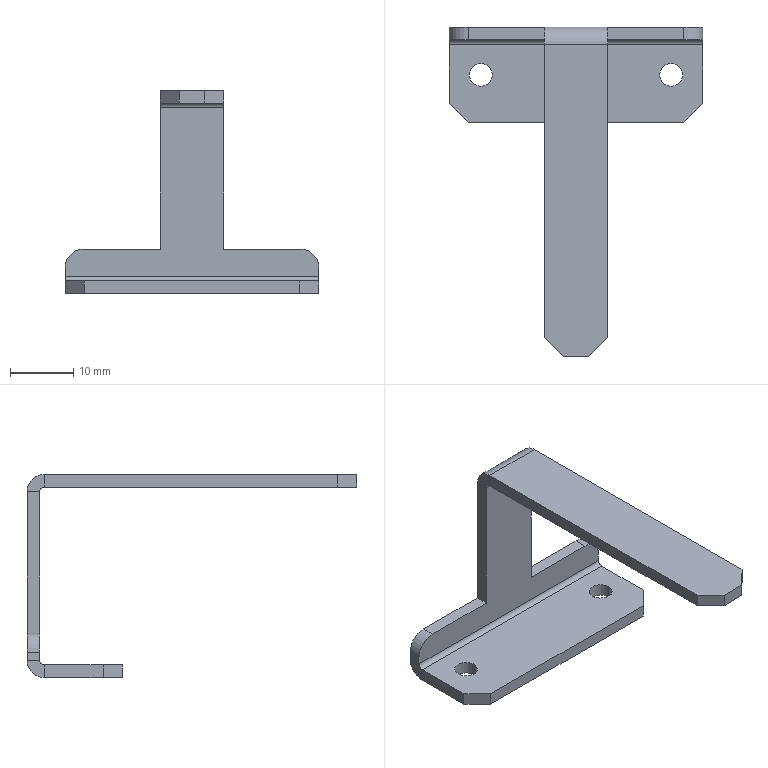Part | SolidWorks | features BaseBody 1 | 1 solid | 36 faces | box 40 x 52 x 32 mm | volume 2941 mm3 | plane 26 | cylinder 10 | commonest cylinder face diameters 3.6 x4 1.473 x2 5.473 x2 6 x2
STEP:
#1=CARTESIAN_POINT('',(-16.8,0.,-2.));
#2=VERTEX_POINT('',#1);
#3=CARTESIAN_POINT('',(-13.2,0.,-2.));
#4=VERTEX_POINT('',#3);
#5=CARTESIAN_POINT('',(-15.,0.,-2.));
#6=DIRECTION('',(0.,0.,1.));
#7=DIRECTION('',(1.,0.,0.));
#8=AXIS2_PLACEMENT_3D('',#5,#6,#7);
#9=CIRCLE('',#8,1.8);
#10=EDGE_CURVE('',#2,#4,#9,.T.);
#11=ORIENTED_EDGE('',*,*,#10,.F.);
#12=CARTESIAN_POINT('',(-16.8,0.,0.));
#13=VERTEX_POINT('',#12);
#14=CARTESIAN_POINT('',(-16.8,0.,0.));
#15=DIRECTION('',(0.,0.,1.));
#16=VECTOR('',#15,1000.);
#17=LINE('',#14,#16);
#18=EDGE_CURVE('',#2,#13,#17,.T.);
#19=ORIENTED_EDGE('',*,*,#18,.T.);
#20=CARTESIAN_POINT('',(-13.2,0.,0.));
#21=VERTEX_POINT('',#20);
#22=CARTESIAN_POINT('',(-15.,0.,0.));
#23=DIRECTION('',(0.,0.,1.));
#24=DIRECTION('',(1.,0.,0.));
#25=AXIS2_PLACEMENT_3D('',#22,#23,#24);
#26=CIRCLE('',#25,1.8);
#27=EDGE_CURVE('',#13,#21,#26,.T.);
#28=ORIENTED_EDGE('',*,*,#27,.T.);
#29=CARTESIAN_POINT('',(-13.2,0.,0.));
#30=DIRECTION('',(0.,0.,1.));
#31=VECTOR('',#30,1000.);
#32=LINE('',#29,#31);
#33=EDGE_CURVE('',#4,#21,#32,.T.);
#34=ORIENTED_EDGE('',*,*,#33,.F.);
#35=EDGE_LOOP('',(#11,#19,#28,#34));
#36=FACE_OUTER_BOUND('',#35,.T.);
#37=CARTESIAN_POINT('',(-15.,0.,0.));
#38=DIRECTION('',(0.,0.,1.));
#39=DIRECTION('',(1.,0.,0.));
#40=AXIS2_PLACEMENT_3D('',#37,#38,#39);
#41=CYLINDRICAL_SURFACE('',#40,1.8);
#42=ADVANCED_FACE('',(#36),#41,.F.);
#43=CARTESIAN_POINT('',(13.2,0.,-2.));
#44=VERTEX_POINT('',#43);
#45=CARTESIAN_POINT('',(16.8,0.,-2.));
#46=VERTEX_POINT('',#45);
#47=CARTESIAN_POINT('',(15.,0.,-2.));
#48=DIRECTION('',(0.,0.,1.));
#49=DIRECTION('',(1.,0.,0.));
#50=AXIS2_PLACEMENT_3D('',#47,#48,#49);
#51=CIRCLE('',#50,1.8);
#52=EDGE_CURVE('',#44,#46,#51,.T.);
#53=ORIENTED_EDGE('',*,*,#52,.F.);
#54=CARTESIAN_POINT('',(13.2,0.,0.));
#55=VERTEX_POINT('',#54);
#56=CARTESIAN_POINT('',(13.2,0.,0.));
#57=DIRECTION('',(0.,0.,1.));
#58=VECTOR('',#57,1000.);
#59=LINE('',#56,#58);
#60=EDGE_CURVE('',#44,#55,#59,.T.);
#61=ORIENTED_EDGE('',*,*,#60,.T.);
#62=CARTESIAN_POINT('',(16.8,0.,0.));
#63=VERTEX_POINT('',#62);
#64=CARTESIAN_POINT('',(15.,0.,0.));
#65=DIRECTION('',(0.,0.,1.));
#66=DIRECTION('',(1.,0.,0.));
#67=AXIS2_PLACEMENT_3D('',#64,#65,#66);
#68=CIRCLE('',#67,1.8);
#69=EDGE_CURVE('',#55,#63,#68,.T.);
#70=ORIENTED_EDGE('',*,*,#69,.T.);
#71=CARTESIAN_POINT('',(16.8,0.,0.));
#72=DIRECTION('',(0.,0.,1.));
#73=VECTOR('',#72,1000.);
#74=LINE('',#71,#73);
#75=EDGE_CURVE('',#46,#63,#74,.T.);
#76=ORIENTED_EDGE('',*,*,#75,.F.);
#77=EDGE_LOOP('',(#53,#61,#70,#76));
#78=FACE_OUTER_BOUND('',#77,.T.);
#79=CARTESIAN_POINT('',(15.,0.,0.));
#80=DIRECTION('',(0.,0.,1.));
#81=DIRECTION('',(1.,0.,0.));
#82=AXIS2_PLACEMENT_3D('',#79,#80,#81);
#83=CYLINDRICAL_SURFACE('',#82,1.8);
#84=ADVANCED_FACE('',(#78),#83,.F.);
#85=CARTESIAN_POINT('',(-5.,4.763,28.));
#86=VERTEX_POINT('',#85);
#87=CARTESIAN_POINT('',(-5.,-41.5,28.));
#88=VERTEX_POINT('',#87);
#89=CARTESIAN_POINT('',(-5.,0.,28.));
#90=DIRECTION('',(0.,-1.,0.));
#91=VECTOR('',#90,1000.);
#92=LINE('',#89,#91);
#93=EDGE_CURVE('',#86,#88,#92,.T.);
#94=ORIENTED_EDGE('',*,*,#93,.T.);
#95=CARTESIAN_POINT('',(-5.,-41.5,30.));
#96=VERTEX_POINT('',#95);
#97=CARTESIAN_POINT('',(-5.,-41.5,5.));
#98=DIRECTION('',(0.,0.,1.));
#99=VECTOR('',#98,1000.);
#100=LINE('',#97,#99);
#101=EDGE_CURVE('',#88,#96,#100,.T.);
#102=ORIENTED_EDGE('',*,*,#101,.T.);
#103=CARTESIAN_POINT('',(-5.,4.763,30.));
#104=VERTEX_POINT('',#103);
#105=CARTESIAN_POINT('',(-5.,-44.5,30.));
#106=DIRECTION('',(0.,-1.,0.));
#107=VECTOR('',#106,1000.);
#108=LINE('',#105,#107);
#109=EDGE_CURVE('',#104,#96,#108,.T.);
#110=ORIENTED_EDGE('',*,*,#109,.F.);
#111=CARTESIAN_POINT('',(-5.,4.763,30.));
#112=DIRECTION('',(0.,0.,-1.));
#113=VECTOR('',#112,1000.);
#114=LINE('',#111,#113);
#115=EDGE_CURVE('',#104,#86,#114,.T.);
#116=ORIENTED_EDGE('',*,*,#115,.T.);
#117=EDGE_LOOP('',(#94,#102,#110,#116));
#118=FACE_OUTER_BOUND('',#117,.T.);
#119=CARTESIAN_POINT('',(-5.,-44.5,5.));
#120=DIRECTION('',(-1.,0.,0.));
#121=DIRECTION('',(0.,-1.,0.));
#122=AXIS2_PLACEMENT_3D('',#119,#120,#121);
#123=PLANE('',#122);
#124=ADVANCED_FACE('',(#118),#123,.T.);
#125=CARTESIAN_POINT('',(-5.,5.5,5.));
#126=VERTEX_POINT('',#125);
#127=CARTESIAN_POINT('',(-5.,5.5,27.263));
#128=VERTEX_POINT('',#127);
#129=CARTESIAN_POINT('',(-5.,5.5,0.));
#130=DIRECTION('',(0.,0.,1.));
#131=VECTOR('',#130,1000.);
#132=LINE('',#129,#131);
#133=EDGE_CURVE('',#126,#128,#132,.T.);
#134=ORIENTED_EDGE('',*,*,#133,.T.);
#135=CARTESIAN_POINT('',(-5.,7.5,27.263));
#136=VERTEX_POINT('',#135);
#137=CARTESIAN_POINT('',(-5.,5.5,27.263));
#138=DIRECTION('',(0.,1.,0.));
#139=VECTOR('',#138,1000.);
#140=LINE('',#137,#139);
#141=EDGE_CURVE('',#128,#136,#140,.T.);
#142=ORIENTED_EDGE('',*,*,#141,.T.);
#143=CARTESIAN_POINT('',(-5.,7.5,5.));
#144=VERTEX_POINT('',#143);
#145=CARTESIAN_POINT('',(-5.,7.5,0.));
#146=DIRECTION('',(0.,0.,1.));
#147=VECTOR('',#146,1000.);
#148=LINE('',#145,#147);
#149=EDGE_CURVE('',#144,#136,#148,.T.);
#150=ORIENTED_EDGE('',*,*,#149,.F.);
#151=CARTESIAN_POINT('',(-5.,-44.5,5.));
#152=DIRECTION('',(0.,-1.,0.));
#153=VECTOR('',#152,1000.);
#154=LINE('',#151,#153);
#155=EDGE_CURVE('',#144,#126,#154,.T.);
#156=ORIENTED_EDGE('',*,*,#155,.T.);
#157=EDGE_LOOP('',(#134,#142,#150,#156));
#158=FACE_OUTER_BOUND('',#157,.T.);
#159=CARTESIAN_POINT('',(-5.,-44.5,5.));
#160=DIRECTION('',(-1.,0.,0.));
#161=DIRECTION('',(0.,-1.,0.));
#162=AXIS2_PLACEMENT_3D('',#159,#160,#161);
#163=PLANE('',#162);
#164=ADVANCED_FACE('',(#158),#163,.T.);
#165=CARTESIAN_POINT('',(5.,-41.5,30.));
#166=VERTEX_POINT('',#165);
#167=CARTESIAN_POINT('',(5.,4.763,30.));
#168=VERTEX_POINT('',#167);
#169=CARTESIAN_POINT('',(5.,-44.5,30.));
#170=DIRECTION('',(0.,1.,0.));
#171=VECTOR('',#170,1000.);
#172=LINE('',#169,#171);
#173=EDGE_CURVE('',#166,#168,#172,.T.);
#174=ORIENTED_EDGE('',*,*,#173,.F.);
#175=CARTESIAN_POINT('',(5.,-41.5,28.));
#176=VERTEX_POINT('',#175);
#177=CARTESIAN_POINT('',(5.,-41.5,5.));
#178=DIRECTION('',(0.,0.,-1.));
#179=VECTOR('',#178,1000.);
#180=LINE('',#177,#179);
#181=EDGE_CURVE('',#166,#176,#180,.T.);
#182=ORIENTED_EDGE('',*,*,#181,.T.);
#183=CARTESIAN_POINT('',(5.,4.763,28.));
#184=VERTEX_POINT('',#183);
#185=CARTESIAN_POINT('',(5.,0.,28.));
#186=DIRECTION('',(0.,1.,0.));
#187=VECTOR('',#186,1000.);
#188=LINE('',#185,#187);
#189=EDGE_CURVE('',#176,#184,#188,.T.);
#190=ORIENTED_EDGE('',*,*,#189,.T.);
#191=CARTESIAN_POINT('',(5.,4.763,28.));
#192=DIRECTION('',(0.,0.,1.));
#193=VECTOR('',#192,1000.);
#194=LINE('',#191,#193);
#195=EDGE_CURVE('',#184,#168,#194,.T.);
#196=ORIENTED_EDGE('',*,*,#195,.T.);
#197=EDGE_LOOP('',(#174,#182,#190,#196));
#198=FACE_OUTER_BOUND('',#197,.T.);
#199=CARTESIAN_POINT('',(5.,-44.5,5.));
#200=DIRECTION('',(1.,0.,0.));
#201=DIRECTION('',(0.,0.,-1.));
#202=AXIS2_PLACEMENT_3D('',#199,#200,#201);
#203=PLANE('',#202);
#204=ADVANCED_FACE('',(#198),#203,.T.);
#205=CARTESIAN_POINT('',(5.,7.5,27.263));
#206=VERTEX_POINT('',#205);
#207=CARTESIAN_POINT('',(5.,7.5,5.));
#208=VERTEX_POINT('',#207);
#209=CARTESIAN_POINT('',(5.,7.5,0.));
#210=DIRECTION('',(0.,0.,-1.));
#211=VECTOR('',#210,1000.);
#212=LINE('',#209,#211);
#213=EDGE_CURVE('',#206,#208,#212,.T.);
#214=ORIENTED_EDGE('',*,*,#213,.F.);
#215=CARTESIAN_POINT('',(5.,5.5,27.263));
#216=VERTEX_POINT('',#215);
#217=CARTESIAN_POINT('',(5.,7.5,27.263));
#218=DIRECTION('',(0.,-1.,0.));
#219=VECTOR('',#218,1000.);
#220=LINE('',#217,#219);
#221=EDGE_CURVE('',#206,#216,#220,.T.);
#222=ORIENTED_EDGE('',*,*,#221,.T.);
#223=CARTESIAN_POINT('',(5.,5.5,5.));
#224=VERTEX_POINT('',#223);
#225=CARTESIAN_POINT('',(5.,5.5,0.));
#226=DIRECTION('',(0.,0.,-1.));
#227=VECTOR('',#226,1000.);
#228=LINE('',#225,#227);
#229=EDGE_CURVE('',#216,#224,#228,.T.);
#230=ORIENTED_EDGE('',*,*,#229,.T.);
#231=CARTESIAN_POINT('',(5.,-44.5,5.));
#232=DIRECTION('',(0.,1.,0.));
#233=VECTOR('',#232,1000.);
#234=LINE('',#231,#233);
#235=EDGE_CURVE('',#224,#208,#234,.T.);
#236=ORIENTED_EDGE('',*,*,#235,.T.);
#237=EDGE_LOOP('',(#214,#222,#230,#236));
#238=FACE_OUTER_BOUND('',#237,.T.);
#239=CARTESIAN_POINT('',(5.,-44.5,5.));
#240=DIRECTION('',(1.,0.,0.));
#241=DIRECTION('',(0.,0.,-1.));
#242=AXIS2_PLACEMENT_3D('',#239,#240,#241);
#243=PLANE('',#242);
#244=ADVANCED_FACE('',(#238),#243,.T.);
#245=CARTESIAN_POINT('',(17.,7.5,5.));
#246=VERTEX_POINT('',#245);
#247=CARTESIAN_POINT('',(0.,7.5,5.));
#248=DIRECTION('',(1.,0.,0.));
#249=VECTOR('',#248,1000.);
#250=LINE('',#247,#249);
#251=EDGE_CURVE('',#208,#246,#250,.T.);
#252=ORIENTED_EDGE('',*,*,#251,.T.);
#253=CARTESIAN_POINT('',(20.,7.5,2.));
#254=VERTEX_POINT('',#253);
#255=CARTESIAN_POINT('',(17.,7.5,2.));
#256=DIRECTION('',(0.,1.,0.));
#257=DIRECTION('',(0.,0.,1.));
#258=AXIS2_PLACEMENT_3D('',#255,#256,#257);
#259=CIRCLE('',#258,3.);
#260=EDGE_CURVE('',#246,#254,#259,.T.);
#261=ORIENTED_EDGE('',*,*,#260,.T.);
#262=CARTESIAN_POINT('',(20.,7.5,0.7366));
#263=VERTEX_POINT('',#262);
#264=CARTESIAN_POINT('',(20.,7.5,28.));
#265=DIRECTION('',(0.,0.,1.));
#266=VECTOR('',#265,1000.);
#267=LINE('',#264,#266);
#268=EDGE_CURVE('',#263,#254,#267,.T.);
#269=ORIENTED_EDGE('',*,*,#268,.F.);
#270=CARTESIAN_POINT('',(-20.,7.5,0.7366));
#271=VERTEX_POINT('',#270);
#272=CARTESIAN_POINT('',(0.,7.5,0.7366));
#273=DIRECTION('',(-1.,0.,0.));
#274=VECTOR('',#273,1000.);
#275=LINE('',#272,#274);
#276=EDGE_CURVE('',#263,#271,#275,.T.);
#277=ORIENTED_EDGE('',*,*,#276,.T.);
#278=CARTESIAN_POINT('',(-20.,7.5,2.));
#279=VERTEX_POINT('',#278);
#280=CARTESIAN_POINT('',(-20.,7.5,0.));
#281=DIRECTION('',(0.,0.,-1.));
#282=VECTOR('',#281,1000.);
#283=LINE('',#280,#282);
#284=EDGE_CURVE('',#279,#271,#283,.T.);
#285=ORIENTED_EDGE('',*,*,#284,.F.);
#286=CARTESIAN_POINT('',(-17.,7.5,5.));
#287=VERTEX_POINT('',#286);
#288=CARTESIAN_POINT('',(-17.,7.5,2.));
#289=DIRECTION('',(0.,1.,0.));
#290=DIRECTION('',(0.,0.,1.));
#291=AXIS2_PLACEMENT_3D('',#288,#289,#290);
#292=CIRCLE('',#291,3.);
#293=EDGE_CURVE('',#279,#287,#292,.T.);
#294=ORIENTED_EDGE('',*,*,#293,.T.);
#295=CARTESIAN_POINT('',(0.,7.5,5.));
#296=DIRECTION('',(1.,0.,0.));
#297=VECTOR('',#296,1000.);
#298=LINE('',#295,#297);
#299=EDGE_CURVE('',#287,#144,#298,.T.);
#300=ORIENTED_EDGE('',*,*,#299,.T.);
#301=ORIENTED_EDGE('',*,*,#149,.T.);
#302=CARTESIAN_POINT('',(-20.,7.5,27.263));
#303=DIRECTION('',(1.,0.,0.));
#304=VECTOR('',#303,1000.);
#305=LINE('',#302,#304);
#306=EDGE_CURVE('',#136,#206,#305,.T.);
#307=ORIENTED_EDGE('',*,*,#306,.T.);
#308=ORIENTED_EDGE('',*,*,#213,.T.);
#309=EDGE_LOOP('',(#252,#261,#269,#277,#285,#294,#300,#301,#307,#308));
#310=FACE_OUTER_BOUND('',#309,.T.);
#311=CARTESIAN_POINT('',(0.,7.5,0.));
#312=DIRECTION('',(0.,1.,0.));
#313=DIRECTION('',(0.,0.,1.));
#314=AXIS2_PLACEMENT_3D('',#311,#312,#313);
#315=PLANE('',#314);
#316=ADVANCED_FACE('',(#310),#315,.T.);
#317=CARTESIAN_POINT('',(20.,5.5,0.7366));
#318=VERTEX_POINT('',#317);
#319=CARTESIAN_POINT('',(20.,5.5,2.));
#320=VERTEX_POINT('',#319);
#321=CARTESIAN_POINT('',(20.,5.5,0.));
#322=DIRECTION('',(0.,0.,1.));
#323=VECTOR('',#322,1000.);
#324=LINE('',#321,#323);
#325=EDGE_CURVE('',#318,#320,#324,.T.);
#326=ORIENTED_EDGE('',*,*,#325,.T.);
#327=CARTESIAN_POINT('',(17.,5.5,5.));
#328=VERTEX_POINT('',#327);
#329=CARTESIAN_POINT('',(17.,5.5,2.));
#330=DIRECTION('',(0.,-1.,0.));
#331=DIRECTION('',(0.,0.,1.));
#332=AXIS2_PLACEMENT_3D('',#329,#330,#331);
#333=CIRCLE('',#332,3.);
#334=EDGE_CURVE('',#320,#328,#333,.T.);
#335=ORIENTED_EDGE('',*,*,#334,.T.);
#336=CARTESIAN_POINT('',(0.,5.5,5.));
#337=DIRECTION('',(1.,0.,0.));
#338=VECTOR('',#337,1000.);
#339=LINE('',#336,#338);
#340=EDGE_CURVE('',#224,#328,#339,.T.);
#341=ORIENTED_EDGE('',*,*,#340,.F.);
#342=ORIENTED_EDGE('',*,*,#229,.F.);
#343=CARTESIAN_POINT('',(-20.,5.5,27.263));
#344=DIRECTION('',(1.,0.,0.));
#345=VECTOR('',#344,1000.);
#346=LINE('',#343,#345);
#347=EDGE_CURVE('',#128,#216,#346,.T.);
#348=ORIENTED_EDGE('',*,*,#347,.F.);
#349=ORIENTED_EDGE('',*,*,#133,.F.);
#350=CARTESIAN_POINT('',(-17.,5.5,5.));
#351=VERTEX_POINT('',#350);
#352=CARTESIAN_POINT('',(0.,5.5,5.));
#353=DIRECTION('',(1.,0.,0.));
#354=VECTOR('',#353,1000.);
#355=LINE('',#352,#354);
#356=EDGE_CURVE('',#351,#126,#355,.T.);
#357=ORIENTED_EDGE('',*,*,#356,.F.);
#358=CARTESIAN_POINT('',(-20.,5.5,2.));
#359=VERTEX_POINT('',#358);
#360=CARTESIAN_POINT('',(-17.,5.5,2.));
#361=DIRECTION('',(0.,-1.,0.));
#362=DIRECTION('',(0.,0.,1.));
#363=AXIS2_PLACEMENT_3D('',#360,#361,#362);
#364=CIRCLE('',#363,3.);
#365=EDGE_CURVE('',#351,#359,#364,.T.);
#366=ORIENTED_EDGE('',*,*,#365,.T.);
#367=CARTESIAN_POINT('',(-20.,5.5,0.7366));
#368=VERTEX_POINT('',#367);
#369=CARTESIAN_POINT('',(-20.,5.5,0.));
#370=DIRECTION('',(0.,0.,-1.));
#371=VECTOR('',#370,1000.);
#372=LINE('',#369,#371);
#373=EDGE_CURVE('',#359,#368,#372,.T.);
#374=ORIENTED_EDGE('',*,*,#373,.T.);
#375=CARTESIAN_POINT('',(20.,5.5,0.7366));
#376=DIRECTION('',(-1.,0.,0.));
#377=VECTOR('',#376,1000.);
#378=LINE('',#375,#377);
#379=EDGE_CURVE('',#318,#368,#378,.T.);
#380=ORIENTED_EDGE('',*,*,#379,.F.);
#381=EDGE_LOOP('',(#326,#335,#341,#342,#348,#349,#357,#366,#374,#380));
#382=FACE_OUTER_BOUND('',#381,.T.);
#383=CARTESIAN_POINT('',(0.,5.5,0.));
#384=DIRECTION('',(0.,1.,0.));
#385=DIRECTION('',(0.,0.,1.));
#386=AXIS2_PLACEMENT_3D('',#383,#384,#385);
#387=PLANE('',#386);
#388=ADVANCED_FACE('',(#382),#387,.F.);
#389=ORIENTED_EDGE('',*,*,#306,.F.);
#390=CARTESIAN_POINT('',(-5.,4.763,27.263));
#391=DIRECTION('',(1.,0.,0.));
#392=DIRECTION('',(0.,-1.,0.));
#393=AXIS2_PLACEMENT_3D('',#390,#391,#392);
#394=CIRCLE('',#393,2.737);
#395=EDGE_CURVE('',#136,#104,#394,.T.);
#396=ORIENTED_EDGE('',*,*,#395,.T.);
#397=CARTESIAN_POINT('',(0.,4.763,30.));
#398=DIRECTION('',(-1.,0.,0.));
#399=VECTOR('',#398,1000.);
#400=LINE('',#397,#399);
#401=EDGE_CURVE('',#168,#104,#400,.T.);
#402=ORIENTED_EDGE('',*,*,#401,.F.);
#403=CARTESIAN_POINT('',(5.,4.763,27.263));
#404=DIRECTION('',(-1.,0.,0.));
#405=DIRECTION('',(0.,0.,-1.));
#406=AXIS2_PLACEMENT_3D('',#403,#404,#405);
#407=CIRCLE('',#406,2.737);
#408=EDGE_CURVE('',#168,#206,#407,.T.);
#409=ORIENTED_EDGE('',*,*,#408,.T.);
#410=EDGE_LOOP('',(#389,#396,#402,#409));
#411=FACE_OUTER_BOUND('',#410,.T.);
#412=CARTESIAN_POINT('',(-20.,4.763,27.263));
#413=DIRECTION('',(-1.,0.,0.));
#414=DIRECTION('',(0.,0.,1.));
#415=AXIS2_PLACEMENT_3D('',#412,#413,#414);
#416=CYLINDRICAL_SURFACE('',#415,2.737);
#417=ADVANCED_FACE('',(#411),#416,.T.);
#418=CARTESIAN_POINT('',(-5.,4.763,27.263));
#419=DIRECTION('',(1.,0.,0.));
#420=DIRECTION('',(0.,-1.,0.));
#421=AXIS2_PLACEMENT_3D('',#418,#419,#420);
#422=CIRCLE('',#421,0.7366);
#423=EDGE_CURVE('',#128,#86,#422,.T.);
#424=ORIENTED_EDGE('',*,*,#423,.F.);
#425=ORIENTED_EDGE('',*,*,#347,.T.);
#426=CARTESIAN_POINT('',(5.,4.763,27.263));
#427=DIRECTION('',(-1.,0.,0.));
#428=DIRECTION('',(0.,0.,-1.));
#429=AXIS2_PLACEMENT_3D('',#426,#427,#428);
#430=CIRCLE('',#429,0.7366);
#431=EDGE_CURVE('',#184,#216,#430,.T.);
#432=ORIENTED_EDGE('',*,*,#431,.F.);
#433=CARTESIAN_POINT('',(20.,4.763,28.));
#434=DIRECTION('',(-1.,0.,0.));
#435=VECTOR('',#434,1000.);
#436=LINE('',#433,#435);
#437=EDGE_CURVE('',#184,#86,#436,.T.);
#438=ORIENTED_EDGE('',*,*,#437,.T.);
#439=EDGE_LOOP('',(#424,#425,#432,#438));
#440=FACE_OUTER_BOUND('',#439,.T.);
#441=CARTESIAN_POINT('',(-20.,4.763,27.263));
#442=DIRECTION('',(-1.,0.,0.));
#443=DIRECTION('',(0.,0.,1.));
#444=AXIS2_PLACEMENT_3D('',#441,#442,#443);
#445=CYLINDRICAL_SURFACE('',#444,0.7366);
#446=ADVANCED_FACE('',(#440),#445,.F.);
#447=CARTESIAN_POINT('',(2.,-44.5,30.));
#448=VERTEX_POINT('',#447);
#449=CARTESIAN_POINT('',(-2.,-44.5,30.));
#450=VERTEX_POINT('',#449);
#451=CARTESIAN_POINT('',(-20.,-44.5,30.));
#452=DIRECTION('',(-1.,0.,0.));
#453=VECTOR('',#452,1000.);
#454=LINE('',#451,#453);
#455=EDGE_CURVE('',#448,#450,#454,.T.);
#456=ORIENTED_EDGE('',*,*,#455,.F.);
#457=CARTESIAN_POINT('',(23.25,-23.25,30.));
#458=DIRECTION('',(0.7071,0.7071,0.));
#459=VECTOR('',#458,1000.);
#460=LINE('',#457,#459);
#461=EDGE_CURVE('',#448,#166,#460,.T.);
#462=ORIENTED_EDGE('',*,*,#461,.T.);
#463=ORIENTED_EDGE('',*,*,#173,.T.);
#464=ORIENTED_EDGE('',*,*,#401,.T.);
#465=ORIENTED_EDGE('',*,*,#109,.T.);
#466=CARTESIAN_POINT('',(-23.25,-23.25,30.));
#467=DIRECTION('',(0.7071,-0.7071,0.));
#468=VECTOR('',#467,1000.);
#469=LINE('',#466,#468);
#470=EDGE_CURVE('',#96,#450,#469,.T.);
#471=ORIENTED_EDGE('',*,*,#470,.T.);
#472=EDGE_LOOP('',(#456,#462,#463,#464,#465,#471));
#473=FACE_OUTER_BOUND('',#472,.T.);
#474=CARTESIAN_POINT('',(0.,0.,30.));
#475=DIRECTION('',(0.,0.,1.));
#476=DIRECTION('',(0.,-1.,0.));
#477=AXIS2_PLACEMENT_3D('',#474,#475,#476);
#478=PLANE('',#477);
#479=ADVANCED_FACE('',(#473),#478,.T.);
#480=ORIENTED_EDGE('',*,*,#189,.F.);
#481=CARTESIAN_POINT('',(2.,-44.5,28.));
#482=VERTEX_POINT('',#481);
#483=CARTESIAN_POINT('',(2.,-44.5,28.));
#484=DIRECTION('',(-0.7071,-0.7071,0.));
#485=VECTOR('',#484,1000.);
#486=LINE('',#483,#485);
#487=EDGE_CURVE('',#176,#482,#486,.T.);
#488=ORIENTED_EDGE('',*,*,#487,.T.);
#489=CARTESIAN_POINT('',(-2.,-44.5,28.));
#490=VERTEX_POINT('',#489);
#491=CARTESIAN_POINT('',(-20.,-44.5,28.));
#492=DIRECTION('',(-1.,0.,0.));
#493=VECTOR('',#492,1000.);
#494=LINE('',#491,#493);
#495=EDGE_CURVE('',#482,#490,#494,.T.);
#496=ORIENTED_EDGE('',*,*,#495,.T.);
#497=CARTESIAN_POINT('',(-5.,-41.5,28.));
#498=DIRECTION('',(-0.7071,0.7071,0.));
#499=VECTOR('',#498,1000.);
#500=LINE('',#497,#499);
#501=EDGE_CURVE('',#490,#88,#500,.T.);
#502=ORIENTED_EDGE('',*,*,#501,.T.);
#503=ORIENTED_EDGE('',*,*,#93,.F.);
#504=ORIENTED_EDGE('',*,*,#437,.F.);
#505=EDGE_LOOP('',(#480,#488,#496,#502,#503,#504));
#506=FACE_OUTER_BOUND('',#505,.T.);
#507=CARTESIAN_POINT('',(0.,0.,28.));
#508=DIRECTION('',(0.,0.,1.));
#509=DIRECTION('',(0.,-1.,0.));
#510=AXIS2_PLACEMENT_3D('',#507,#508,#509);
#511=PLANE('',#510);
#512=ADVANCED_FACE('',(#506),#511,.F.);
#513=ORIENTED_EDGE('',*,*,#495,.F.);
#514=CARTESIAN_POINT('',(2.,-44.5,30.));
#515=DIRECTION('',(0.,0.,1.));
#516=VECTOR('',#515,1000.);
#517=LINE('',#514,#516);
#518=EDGE_CURVE('',#482,#448,#517,.T.);
#519=ORIENTED_EDGE('',*,*,#518,.T.);
#520=ORIENTED_EDGE('',*,*,#455,.T.);
#521=CARTESIAN_POINT('',(-2.,-44.5,30.));
#522=DIRECTION('',(0.,0.,-1.));
#523=VECTOR('',#522,1000.);
#524=LINE('',#521,#523);
#525=EDGE_CURVE('',#450,#490,#524,.T.);
#526=ORIENTED_EDGE('',*,*,#525,.T.);
#527=EDGE_LOOP('',(#513,#519,#520,#526));
#528=FACE_OUTER_BOUND('',#527,.T.);
#529=CARTESIAN_POINT('',(-20.,-44.5,30.));
#530=DIRECTION('',(0.,-1.,0.));
#531=DIRECTION('',(0.,0.,-1.));
#532=AXIS2_PLACEMENT_3D('',#529,#530,#531);
#533=PLANE('',#532);
#534=ADVANCED_FACE('',(#528),#533,.T.);
#535=ORIENTED_EDGE('',*,*,#373,.F.);
#536=CARTESIAN_POINT('',(-20.,7.5,2.));
#537=DIRECTION('',(0.,1.,0.));
#538=VECTOR('',#537,1000.);
#539=LINE('',#536,#538);
#540=EDGE_CURVE('',#359,#279,#539,.T.);
#541=ORIENTED_EDGE('',*,*,#540,.T.);
#542=ORIENTED_EDGE('',*,*,#284,.T.);
#543=CARTESIAN_POINT('',(-20.,5.5,0.7366));
#544=DIRECTION('',(0.,1.,0.));
#545=VECTOR('',#544,1000.);
#546=LINE('',#543,#545);
#547=EDGE_CURVE('',#368,#271,#546,.T.);
#548=ORIENTED_EDGE('',*,*,#547,.F.);
#549=EDGE_LOOP('',(#535,#541,#542,#548));
#550=FACE_OUTER_BOUND('',#549,.T.);
#551=CARTESIAN_POINT('',(-20.,7.5,0.));
#552=DIRECTION('',(-1.,0.,0.));
#553=DIRECTION('',(0.,-1.,0.));
#554=AXIS2_PLACEMENT_3D('',#551,#552,#553);
#555=PLANE('',#554);
#556=ADVANCED_FACE('',(#550),#555,.T.);
#557=ORIENTED_EDGE('',*,*,#268,.T.);
#558=CARTESIAN_POINT('',(20.,7.5,2.));
#559=DIRECTION('',(0.,-1.,0.));
#560=VECTOR('',#559,1000.);
#561=LINE('',#558,#560);
#562=EDGE_CURVE('',#254,#320,#561,.T.);
#563=ORIENTED_EDGE('',*,*,#562,.T.);
#564=ORIENTED_EDGE('',*,*,#325,.F.);
#565=CARTESIAN_POINT('',(20.,7.5,0.7366));
#566=DIRECTION('',(0.,1.,0.));
#567=VECTOR('',#566,1000.);
#568=LINE('',#565,#567);
#569=EDGE_CURVE('',#318,#263,#568,.T.);
#570=ORIENTED_EDGE('',*,*,#569,.T.);
#571=EDGE_LOOP('',(#557,#563,#564,#570));
#572=FACE_OUTER_BOUND('',#571,.T.);
#573=CARTESIAN_POINT('',(20.,7.5,28.));
#574=DIRECTION('',(1.,0.,0.));
#575=DIRECTION('',(0.,1.,0.));
#576=AXIS2_PLACEMENT_3D('',#573,#574,#575);
#577=PLANE('',#576);
#578=ADVANCED_FACE('',(#572),#577,.T.);
#579=CARTESIAN_POINT('',(-20.,4.763,-2.));
#580=VERTEX_POINT('',#579);
#581=CARTESIAN_POINT('',(-20.,-4.5,-2.));
#582=VERTEX_POINT('',#581);
#583=CARTESIAN_POINT('',(-20.,-7.5,-2.));
#584=DIRECTION('',(0.,-1.,0.));
#585=VECTOR('',#584,1000.);
#586=LINE('',#583,#585);
#587=EDGE_CURVE('',#580,#582,#586,.T.);
#588=ORIENTED_EDGE('',*,*,#587,.T.);
#589=CARTESIAN_POINT('',(-20.,-4.5,0.));
#590=VERTEX_POINT('',#589);
#591=CARTESIAN_POINT('',(-20.,-4.5,-2.));
#592=DIRECTION('',(0.,0.,1.));
#593=VECTOR('',#592,1000.);
#594=LINE('',#591,#593);
#595=EDGE_CURVE('',#582,#590,#594,.T.);
#596=ORIENTED_EDGE('',*,*,#595,.T.);
#597=CARTESIAN_POINT('',(-20.,4.763,0.));
#598=VERTEX_POINT('',#597);
#599=CARTESIAN_POINT('',(-20.,-7.5,0.));
#600=DIRECTION('',(0.,-1.,0.));
#601=VECTOR('',#600,1000.);
#602=LINE('',#599,#601);
#603=EDGE_CURVE('',#598,#590,#602,.T.);
#604=ORIENTED_EDGE('',*,*,#603,.F.);
#605=CARTESIAN_POINT('',(-20.,4.763,0.));
#606=DIRECTION('',(0.,0.,-1.));
#607=VECTOR('',#606,1000.);
#608=LINE('',#605,#607);
#609=EDGE_CURVE('',#598,#580,#608,.T.);
#610=ORIENTED_EDGE('',*,*,#609,.T.);
#611=EDGE_LOOP('',(#588,#596,#604,#610));
#612=FACE_OUTER_BOUND('',#611,.T.);
#613=CARTESIAN_POINT('',(-20.,-7.5,-2.));
#614=DIRECTION('',(-1.,0.,0.));
#615=DIRECTION('',(0.,0.,1.));
#616=AXIS2_PLACEMENT_3D('',#613,#614,#615);
#617=PLANE('',#616);
#618=ADVANCED_FACE('',(#612),#617,.T.);
#619=CARTESIAN_POINT('',(-15.,0.,-2.));
#620=DIRECTION('',(0.,0.,1.));
#621=DIRECTION('',(1.,0.,0.));
#622=AXIS2_PLACEMENT_3D('',#619,#620,#621);
#623=CIRCLE('',#622,1.8);
#624=EDGE_CURVE('',#4,#2,#623,.T.);
#625=ORIENTED_EDGE('',*,*,#624,.T.);
#626=ORIENTED_EDGE('',*,*,#10,.T.);
#627=EDGE_LOOP('',(#625,#626));
#628=FACE_BOUND('',#627,.T.);
#629=CARTESIAN_POINT('',(15.,0.,-2.));
#630=DIRECTION('',(0.,0.,1.));
#631=DIRECTION('',(1.,0.,0.));
#632=AXIS2_PLACEMENT_3D('',#629,#630,#631);
#633=CIRCLE('',#632,1.8);
#634=EDGE_CURVE('',#46,#44,#633,.T.);
#635=ORIENTED_EDGE('',*,*,#634,.T.);
#636=ORIENTED_EDGE('',*,*,#52,.T.);
#637=EDGE_LOOP('',(#635,#636));
#638=FACE_BOUND('',#637,.T.);
#639=CARTESIAN_POINT('',(-17.,-7.5,-2.));
#640=VERTEX_POINT('',#639);
#641=CARTESIAN_POINT('',(17.,-7.5,-2.));
#642=VERTEX_POINT('',#641);
#643=CARTESIAN_POINT('',(20.,-7.5,-2.));
#644=DIRECTION('',(1.,0.,0.));
#645=VECTOR('',#644,1000.);
#646=LINE('',#643,#645);
#647=EDGE_CURVE('',#640,#642,#646,.T.);
#648=ORIENTED_EDGE('',*,*,#647,.F.);
#649=CARTESIAN_POINT('',(-20.,-4.5,-2.));
#650=DIRECTION('',(-0.7071,0.7071,0.));
#651=VECTOR('',#650,1000.);
#652=LINE('',#649,#651);
#653=EDGE_CURVE('',#640,#582,#652,.T.);
#654=ORIENTED_EDGE('',*,*,#653,.T.);
#655=ORIENTED_EDGE('',*,*,#587,.F.);
#656=CARTESIAN_POINT('',(20.,4.763,-2.));
#657=VERTEX_POINT('',#656);
#658=CARTESIAN_POINT('',(-20.,4.763,-2.));
#659=DIRECTION('',(1.,0.,0.));
#660=VECTOR('',#659,1000.);
#661=LINE('',#658,#660);
#662=EDGE_CURVE('',#580,#657,#661,.T.);
#663=ORIENTED_EDGE('',*,*,#662,.T.);
#664=CARTESIAN_POINT('',(20.,-4.5,-2.));
#665=VERTEX_POINT('',#664);
#666=CARTESIAN_POINT('',(20.,-7.5,-2.));
#667=DIRECTION('',(0.,1.,0.));
#668=VECTOR('',#667,1000.);
#669=LINE('',#666,#668);
#670=EDGE_CURVE('',#665,#657,#669,.T.);
#671=ORIENTED_EDGE('',*,*,#670,.F.);
#672=CARTESIAN_POINT('',(17.,-7.5,-2.));
#673=DIRECTION('',(-0.7071,-0.7071,0.));
#674=VECTOR('',#673,1000.);
#675=LINE('',#672,#674);
#676=EDGE_CURVE('',#665,#642,#675,.T.);
#677=ORIENTED_EDGE('',*,*,#676,.T.);
#678=EDGE_LOOP('',(#648,#654,#655,#663,#671,#677));
#679=FACE_OUTER_BOUND('',#678,.T.);
#680=CARTESIAN_POINT('',(0.,0.,-2.));
#681=DIRECTION('',(0.,0.,1.));
#682=DIRECTION('',(1.,0.,0.));
#683=AXIS2_PLACEMENT_3D('',#680,#681,#682);
#684=PLANE('',#683);
#685=ADVANCED_FACE('',(#628,#638,#679),#684,.F.);
#686=CARTESIAN_POINT('',(-15.,0.,0.));
#687=DIRECTION('',(0.,0.,1.));
#688=DIRECTION('',(1.,0.,0.));
#689=AXIS2_PLACEMENT_3D('',#686,#687,#688);
#690=CIRCLE('',#689,1.8);
#691=EDGE_CURVE('',#21,#13,#690,.T.);
#692=ORIENTED_EDGE('',*,*,#691,.F.);
#693=ORIENTED_EDGE('',*,*,#27,.F.);
#694=EDGE_LOOP('',(#692,#693));
#695=FACE_BOUND('',#694,.T.);
#696=CARTESIAN_POINT('',(15.,0.,0.));
#697=DIRECTION('',(0.,0.,1.));
#698=DIRECTION('',(1.,0.,0.));
#699=AXIS2_PLACEMENT_3D('',#696,#697,#698);
#700=CIRCLE('',#699,1.8);
#701=EDGE_CURVE('',#63,#55,#700,.T.);
#702=ORIENTED_EDGE('',*,*,#701,.F.);
#703=ORIENTED_EDGE('',*,*,#69,.F.);
#704=EDGE_LOOP('',(#702,#703));
#705=FACE_BOUND('',#704,.T.);
#706=ORIENTED_EDGE('',*,*,#603,.T.);
#707=CARTESIAN_POINT('',(-17.,-7.5,0.));
#708=VERTEX_POINT('',#707);
#709=CARTESIAN_POINT('',(-12.25,-12.25,0.));
#710=DIRECTION('',(0.7071,-0.7071,0.));
#711=VECTOR('',#710,1000.);
#712=LINE('',#709,#711);
#713=EDGE_CURVE('',#590,#708,#712,.T.);
#714=ORIENTED_EDGE('',*,*,#713,.T.);
#715=CARTESIAN_POINT('',(17.,-7.5,0.));
#716=VERTEX_POINT('',#715);
#717=CARTESIAN_POINT('',(20.,-7.5,0.));
#718=DIRECTION('',(1.,0.,0.));
#719=VECTOR('',#718,1000.);
#720=LINE('',#717,#719);
#721=EDGE_CURVE('',#708,#716,#720,.T.);
#722=ORIENTED_EDGE('',*,*,#721,.T.);
#723=CARTESIAN_POINT('',(20.,-4.5,0.));
#724=VERTEX_POINT('',#723);
#725=CARTESIAN_POINT('',(12.25,-12.25,0.));
#726=DIRECTION('',(0.7071,0.7071,0.));
#727=VECTOR('',#726,1000.);
#728=LINE('',#725,#727);
#729=EDGE_CURVE('',#716,#724,#728,.T.);
#730=ORIENTED_EDGE('',*,*,#729,.T.);
#731=CARTESIAN_POINT('',(20.,4.763,0.));
#732=VERTEX_POINT('',#731);
#733=CARTESIAN_POINT('',(20.,-7.5,0.));
#734=DIRECTION('',(0.,1.,0.));
#735=VECTOR('',#734,1000.);
#736=LINE('',#733,#735);
#737=EDGE_CURVE('',#724,#732,#736,.T.);
#738=ORIENTED_EDGE('',*,*,#737,.T.);
#739=CARTESIAN_POINT('',(-20.,4.763,0.));
#740=DIRECTION('',(1.,0.,0.));
#741=VECTOR('',#740,1000.);
#742=LINE('',#739,#741);
#743=EDGE_CURVE('',#598,#732,#742,.T.);
#744=ORIENTED_EDGE('',*,*,#743,.F.);
#745=EDGE_LOOP('',(#706,#714,#722,#730,#738,#744));
#746=FACE_OUTER_BOUND('',#745,.T.);
#747=CARTESIAN_POINT('',(0.,0.,0.));
#748=DIRECTION('',(0.,0.,1.));
#749=DIRECTION('',(1.,0.,0.));
#750=AXIS2_PLACEMENT_3D('',#747,#748,#749);
#751=PLANE('',#750);
#752=ADVANCED_FACE('',(#695,#705,#746),#751,.T.);
#753=ORIENTED_EDGE('',*,*,#737,.F.);
#754=CARTESIAN_POINT('',(20.,-4.5,-2.));
#755=DIRECTION('',(0.,0.,-1.));
#756=VECTOR('',#755,1000.);
#757=LINE('',#754,#756);
#758=EDGE_CURVE('',#724,#665,#757,.T.);
#759=ORIENTED_EDGE('',*,*,#758,.T.);
#760=ORIENTED_EDGE('',*,*,#670,.T.);
#761=CARTESIAN_POINT('',(20.,4.763,0.));
#762=DIRECTION('',(0.,0.,-1.));
#763=VECTOR('',#762,1000.);
#764=LINE('',#761,#763);
#765=EDGE_CURVE('',#732,#657,#764,.T.);
#766=ORIENTED_EDGE('',*,*,#765,.F.);
#767=EDGE_LOOP('',(#753,#759,#760,#766));
#768=FACE_OUTER_BOUND('',#767,.T.);
#769=CARTESIAN_POINT('',(20.,-7.5,-2.));
#770=DIRECTION('',(1.,0.,0.));
#771=DIRECTION('',(0.,0.,-1.));
#772=AXIS2_PLACEMENT_3D('',#769,#770,#771);
#773=PLANE('',#772);
#774=ADVANCED_FACE('',(#768),#773,.T.);
#775=ORIENTED_EDGE('',*,*,#721,.F.);
#776=CARTESIAN_POINT('',(-17.,-7.5,-2.));
#777=DIRECTION('',(0.,0.,-1.));
#778=VECTOR('',#777,1000.);
#779=LINE('',#776,#778);
#780=EDGE_CURVE('',#708,#640,#779,.T.);
#781=ORIENTED_EDGE('',*,*,#780,.T.);
#782=ORIENTED_EDGE('',*,*,#647,.T.);
#783=CARTESIAN_POINT('',(17.,-7.5,-2.));
#784=DIRECTION('',(0.,0.,1.));
#785=VECTOR('',#784,1000.);
#786=LINE('',#783,#785);
#787=EDGE_CURVE('',#642,#716,#786,.T.);
#788=ORIENTED_EDGE('',*,*,#787,.T.);
#789=EDGE_LOOP('',(#775,#781,#782,#788));
#790=FACE_OUTER_BOUND('',#789,.T.);
#791=CARTESIAN_POINT('',(20.,-7.5,-2.));
#792=DIRECTION('',(0.,-1.,0.));
#793=DIRECTION('',(1.,0.,0.));
#794=AXIS2_PLACEMENT_3D('',#791,#792,#793);
#795=PLANE('',#794);
#796=ADVANCED_FACE('',(#790),#795,.T.);
#797=ORIENTED_EDGE('',*,*,#569,.F.);
#798=CARTESIAN_POINT('',(20.,4.763,0.7366));
#799=DIRECTION('',(1.,0.,0.));
#800=DIRECTION('',(0.,0.,1.));
#801=AXIS2_PLACEMENT_3D('',#798,#799,#800);
#802=CIRCLE('',#801,0.7366);
#803=EDGE_CURVE('',#732,#318,#802,.T.);
#804=ORIENTED_EDGE('',*,*,#803,.F.);
#805=ORIENTED_EDGE('',*,*,#765,.T.);
#806=CARTESIAN_POINT('',(20.,4.763,0.7366));
#807=DIRECTION('',(1.,0.,0.));
#808=DIRECTION('',(0.,0.,1.));
#809=AXIS2_PLACEMENT_3D('',#806,#807,#808);
#810=CIRCLE('',#809,2.737);
#811=EDGE_CURVE('',#657,#263,#810,.T.);
#812=ORIENTED_EDGE('',*,*,#811,.T.);
#813=EDGE_LOOP('',(#797,#804,#805,#812));
#814=FACE_OUTER_BOUND('',#813,.T.);
#815=CARTESIAN_POINT('',(20.,4.763,0.7366));
#816=DIRECTION('',(1.,0.,0.));
#817=DIRECTION('',(0.,0.,-1.));
#818=AXIS2_PLACEMENT_3D('',#815,#816,#817);
#819=PLANE('',#818);
#820=ADVANCED_FACE('',(#814),#819,.T.);
#821=CARTESIAN_POINT('',(-20.,4.763,0.7366));
#822=DIRECTION('',(-1.,0.,0.));
#823=DIRECTION('',(0.,0.,1.));
#824=AXIS2_PLACEMENT_3D('',#821,#822,#823);
#825=CIRCLE('',#824,0.7366);
#826=EDGE_CURVE('',#368,#598,#825,.T.);
#827=ORIENTED_EDGE('',*,*,#826,.F.);
#828=ORIENTED_EDGE('',*,*,#547,.T.);
#829=CARTESIAN_POINT('',(-20.,4.763,0.7366));
#830=DIRECTION('',(-1.,0.,0.));
#831=DIRECTION('',(0.,0.,1.));
#832=AXIS2_PLACEMENT_3D('',#829,#830,#831);
#833=CIRCLE('',#832,2.737);
#834=EDGE_CURVE('',#271,#580,#833,.T.);
#835=ORIENTED_EDGE('',*,*,#834,.T.);
#836=ORIENTED_EDGE('',*,*,#609,.F.);
#837=EDGE_LOOP('',(#827,#828,#835,#836));
#838=FACE_OUTER_BOUND('',#837,.T.);
#839=CARTESIAN_POINT('',(-20.,4.763,0.7366));
#840=DIRECTION('',(1.,0.,0.));
#841=DIRECTION('',(0.,0.,-1.));
#842=AXIS2_PLACEMENT_3D('',#839,#840,#841);
#843=PLANE('',#842);
#844=ADVANCED_FACE('',(#838),#843,.F.);
#845=ORIENTED_EDGE('',*,*,#662,.F.);
#846=ORIENTED_EDGE('',*,*,#834,.F.);
#847=ORIENTED_EDGE('',*,*,#276,.F.);
#848=ORIENTED_EDGE('',*,*,#811,.F.);
#849=EDGE_LOOP('',(#845,#846,#847,#848));
#850=FACE_OUTER_BOUND('',#849,.T.);
#851=CARTESIAN_POINT('',(-20.,4.763,0.7366));
#852=DIRECTION('',(-1.,0.,0.));
#853=DIRECTION('',(0.,1.,0.));
#854=AXIS2_PLACEMENT_3D('',#851,#852,#853);
#855=CYLINDRICAL_SURFACE('',#854,2.737);
#856=ADVANCED_FACE('',(#850),#855,.T.);
#857=ORIENTED_EDGE('',*,*,#743,.T.);
#858=ORIENTED_EDGE('',*,*,#803,.T.);
#859=ORIENTED_EDGE('',*,*,#379,.T.);
#860=ORIENTED_EDGE('',*,*,#826,.T.);
#861=EDGE_LOOP('',(#857,#858,#859,#860));
#862=FACE_OUTER_BOUND('',#861,.T.);
#863=CARTESIAN_POINT('',(-20.,4.763,0.7366));
#864=DIRECTION('',(-1.,0.,0.));
#865=DIRECTION('',(0.,1.,0.));
#866=AXIS2_PLACEMENT_3D('',#863,#864,#865);
#867=CYLINDRICAL_SURFACE('',#866,0.7366);
#868=ADVANCED_FACE('',(#862),#867,.F.);
#869=ORIENTED_EDGE('',*,*,#340,.T.);
#870=CARTESIAN_POINT('',(17.,0.,5.));
#871=DIRECTION('',(0.,1.,0.));
#872=VECTOR('',#871,1000.);
#873=LINE('',#870,#872);
#874=EDGE_CURVE('',#328,#246,#873,.T.);
#875=ORIENTED_EDGE('',*,*,#874,.T.);
#876=ORIENTED_EDGE('',*,*,#251,.F.);
#877=ORIENTED_EDGE('',*,*,#235,.F.);
#878=EDGE_LOOP('',(#869,#875,#876,#877));
#879=FACE_OUTER_BOUND('',#878,.T.);
#880=CARTESIAN_POINT('',(0.,0.,5.));
#881=DIRECTION('',(0.,0.,1.));
#882=DIRECTION('',(1.,0.,0.));
#883=AXIS2_PLACEMENT_3D('',#880,#881,#882);
#884=PLANE('',#883);
#885=ADVANCED_FACE('',(#879),#884,.T.);
#886=ORIENTED_EDGE('',*,*,#195,.F.);
#887=ORIENTED_EDGE('',*,*,#431,.T.);
#888=ORIENTED_EDGE('',*,*,#221,.F.);
#889=ORIENTED_EDGE('',*,*,#408,.F.);
#890=EDGE_LOOP('',(#886,#887,#888,#889));
#891=FACE_OUTER_BOUND('',#890,.T.);
#892=CARTESIAN_POINT('',(5.,-44.5,5.));
#893=DIRECTION('',(1.,0.,0.));
#894=DIRECTION('',(0.,0.,-1.));
#895=AXIS2_PLACEMENT_3D('',#892,#893,#894);
#896=PLANE('',#895);
#897=ADVANCED_FACE('',(#891),#896,.T.);
#898=ORIENTED_EDGE('',*,*,#115,.F.);
#899=ORIENTED_EDGE('',*,*,#395,.F.);
#900=ORIENTED_EDGE('',*,*,#141,.F.);
#901=ORIENTED_EDGE('',*,*,#423,.T.);
#902=EDGE_LOOP('',(#898,#899,#900,#901));
#903=FACE_OUTER_BOUND('',#902,.T.);
#904=CARTESIAN_POINT('',(-5.,-44.5,5.));
#905=DIRECTION('',(-1.,0.,0.));
#906=DIRECTION('',(0.,-1.,0.));
#907=AXIS2_PLACEMENT_3D('',#904,#905,#906);
#908=PLANE('',#907);
#909=ADVANCED_FACE('',(#903),#908,.T.);
#910=ORIENTED_EDGE('',*,*,#299,.F.);
#911=CARTESIAN_POINT('',(-17.,0.,5.));
#912=DIRECTION('',(0.,-1.,0.));
#913=VECTOR('',#912,1000.);
#914=LINE('',#911,#913);
#915=EDGE_CURVE('',#287,#351,#914,.T.);
#916=ORIENTED_EDGE('',*,*,#915,.T.);
#917=ORIENTED_EDGE('',*,*,#356,.T.);
#918=ORIENTED_EDGE('',*,*,#155,.F.);
#919=EDGE_LOOP('',(#910,#916,#917,#918));
#920=FACE_OUTER_BOUND('',#919,.T.);
#921=CARTESIAN_POINT('',(0.,0.,5.));
#922=DIRECTION('',(0.,0.,1.));
#923=DIRECTION('',(1.,0.,0.));
#924=AXIS2_PLACEMENT_3D('',#921,#922,#923);
#925=PLANE('',#924);
#926=ADVANCED_FACE('',(#920),#925,.T.);
#927=ORIENTED_EDGE('',*,*,#487,.F.);
#928=ORIENTED_EDGE('',*,*,#181,.F.);
#929=ORIENTED_EDGE('',*,*,#461,.F.);
#930=ORIENTED_EDGE('',*,*,#518,.F.);
#931=EDGE_LOOP('',(#927,#928,#929,#930));
#932=FACE_OUTER_BOUND('',#931,.T.);
#933=CARTESIAN_POINT('',(2.,-44.5,30.));
#934=DIRECTION('',(-0.7071,0.7071,0.));
#935=DIRECTION('',(0.,0.,1.));
#936=AXIS2_PLACEMENT_3D('',#933,#934,#935);
#937=PLANE('',#936);
#938=ADVANCED_FACE('',(#932),#937,.F.);
#939=ORIENTED_EDGE('',*,*,#501,.F.);
#940=ORIENTED_EDGE('',*,*,#525,.F.);
#941=ORIENTED_EDGE('',*,*,#470,.F.);
#942=ORIENTED_EDGE('',*,*,#101,.F.);
#943=EDGE_LOOP('',(#939,#940,#941,#942));
#944=FACE_OUTER_BOUND('',#943,.T.);
#945=CARTESIAN_POINT('',(-5.,-41.5,5.));
#946=DIRECTION('',(0.7071,0.7071,0.));
#947=DIRECTION('',(0.,0.,1.));
#948=AXIS2_PLACEMENT_3D('',#945,#946,#947);
#949=PLANE('',#948);
#950=ADVANCED_FACE('',(#944),#949,.F.);
#951=ORIENTED_EDGE('',*,*,#653,.F.);
#952=ORIENTED_EDGE('',*,*,#780,.F.);
#953=ORIENTED_EDGE('',*,*,#713,.F.);
#954=ORIENTED_EDGE('',*,*,#595,.F.);
#955=EDGE_LOOP('',(#951,#952,#953,#954));
#956=FACE_OUTER_BOUND('',#955,.T.);
#957=CARTESIAN_POINT('',(-20.,-4.5,-2.));
#958=DIRECTION('',(0.7071,0.7071,0.));
#959=DIRECTION('',(0.,0.,1.));
#960=AXIS2_PLACEMENT_3D('',#957,#958,#959);
#961=PLANE('',#960);
#962=ADVANCED_FACE('',(#956),#961,.F.);
#963=ORIENTED_EDGE('',*,*,#676,.F.);
#964=ORIENTED_EDGE('',*,*,#758,.F.);
#965=ORIENTED_EDGE('',*,*,#729,.F.);
#966=ORIENTED_EDGE('',*,*,#787,.F.);
#967=EDGE_LOOP('',(#963,#964,#965,#966));
#968=FACE_OUTER_BOUND('',#967,.T.);
#969=CARTESIAN_POINT('',(17.,-7.5,-2.));
#970=DIRECTION('',(-0.7071,0.7071,0.));
#971=DIRECTION('',(0.,0.,1.));
#972=AXIS2_PLACEMENT_3D('',#969,#970,#971);
#973=PLANE('',#972);
#974=ADVANCED_FACE('',(#968),#973,.F.);
#975=ORIENTED_EDGE('',*,*,#60,.F.);
#976=ORIENTED_EDGE('',*,*,#634,.F.);
#977=ORIENTED_EDGE('',*,*,#75,.T.);
#978=ORIENTED_EDGE('',*,*,#701,.T.);
#979=EDGE_LOOP('',(#975,#976,#977,#978));
#980=FACE_OUTER_BOUND('',#979,.T.);
#981=CARTESIAN_POINT('',(15.,0.,0.));
#982=DIRECTION('',(0.,0.,1.));
#983=DIRECTION('',(1.,0.,0.));
#984=AXIS2_PLACEMENT_3D('',#981,#982,#983);
#985=CYLINDRICAL_SURFACE('',#984,1.8);
#986=ADVANCED_FACE('',(#980),#985,.F.);
#987=ORIENTED_EDGE('',*,*,#18,.F.);
#988=ORIENTED_EDGE('',*,*,#624,.F.);
#989=ORIENTED_EDGE('',*,*,#33,.T.);
#990=ORIENTED_EDGE('',*,*,#691,.T.);
#991=EDGE_LOOP('',(#987,#988,#989,#990));
#992=FACE_OUTER_BOUND('',#991,.T.);
#993=CARTESIAN_POINT('',(-15.,0.,0.));
#994=DIRECTION('',(0.,0.,1.));
#995=DIRECTION('',(1.,0.,0.));
#996=AXIS2_PLACEMENT_3D('',#993,#994,#995);
#997=CYLINDRICAL_SURFACE('',#996,1.8);
#998=ADVANCED_FACE('',(#992),#997,.F.);
#999=ORIENTED_EDGE('',*,*,#260,.F.);
#1000=ORIENTED_EDGE('',*,*,#874,.F.);
#1001=ORIENTED_EDGE('',*,*,#334,.F.);
#1002=ORIENTED_EDGE('',*,*,#562,.F.);
#1003=EDGE_LOOP('',(#999,#1000,#1001,#1002));
#1004=FACE_OUTER_BOUND('',#1003,.T.);
#1005=CARTESIAN_POINT('',(17.,7.5,2.));
#1006=DIRECTION('',(0.,-1.,0.));
#1007=DIRECTION('',(1.,0.,0.));
#1008=AXIS2_PLACEMENT_3D('',#1005,#1006,#1007);
#1009=CYLINDRICAL_SURFACE('',#1008,3.);
#1010=ADVANCED_FACE('',(#1004),#1009,.T.);
#1011=ORIENTED_EDGE('',*,*,#365,.F.);
#1012=ORIENTED_EDGE('',*,*,#915,.F.);
#1013=ORIENTED_EDGE('',*,*,#293,.F.);
#1014=ORIENTED_EDGE('',*,*,#540,.F.);
#1015=EDGE_LOOP('',(#1011,#1012,#1013,#1014));
#1016=FACE_OUTER_BOUND('',#1015,.T.);
#1017=CARTESIAN_POINT('',(-17.,7.5,2.));
#1018=DIRECTION('',(0.,1.,0.));
#1019=DIRECTION('',(-1.,0.,0.));
#1020=AXIS2_PLACEMENT_3D('',#1017,#1018,#1019);
#1021=CYLINDRICAL_SURFACE('',#1020,3.);
#1022=ADVANCED_FACE('',(#1016),#1021,.T.);
#1023=CLOSED_SHELL('',(#42,#84,#124,#164,#204,#244,#316,#388,#417,#446,#479,#512,#534,#556,#578,#618,#685,#752,#774,#796,#820,#844,#856,#868,#885,#897,#909,#926,#938,#950,#962,#974,#986,#998,#1010,#1022));
#1024=MANIFOLD_SOLID_BREP('',#1023);
#1025=CARTESIAN_POINT('',(0.,0.,0.));
#1026=DIRECTION('',(0.,0.,1.));
#1027=DIRECTION('',(1.,0.,0.));
#1028=AXIS2_PLACEMENT_3D('',#1025,#1026,#1027);
#1029=(LENGTH_UNIT()NAMED_UNIT(*)SI_UNIT(.MILLI.,.METRE.));
#1030=UNCERTAINTY_MEASURE_WITH_UNIT(LENGTH_MEASURE(0.00001),#1029,'','');
#1031=(NAMED_UNIT(*)PLANE_ANGLE_UNIT()SI_UNIT($,.RADIAN.));
#1032=(NAMED_UNIT(*)SI_UNIT($,.STERADIAN.)SOLID_ANGLE_UNIT());
#1033=(GEOMETRIC_REPRESENTATION_CONTEXT(3)GLOBAL_UNCERTAINTY_ASSIGNED_CONTEXT((#1030))GLOBAL_UNIT_ASSIGNED_CONTEXT((#1029,#1031,#1032))REPRESENTATION_CONTEXT('',''));
#1034=ADVANCED_BREP_SHAPE_REPRESENTATION('',(#1024,#1028),#1033);